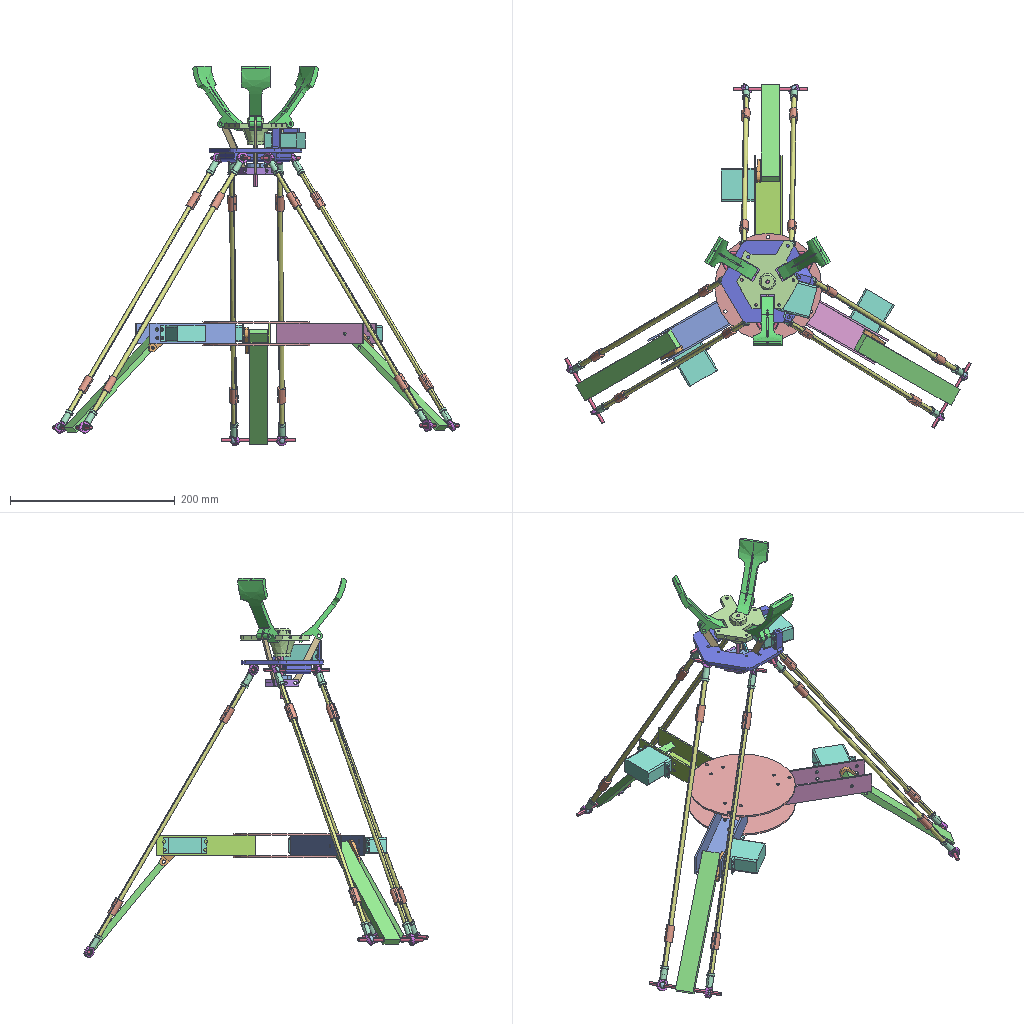Assembly | SolidWorks | 21 different items | 85 placed | box 494 x 418 x 460 mm
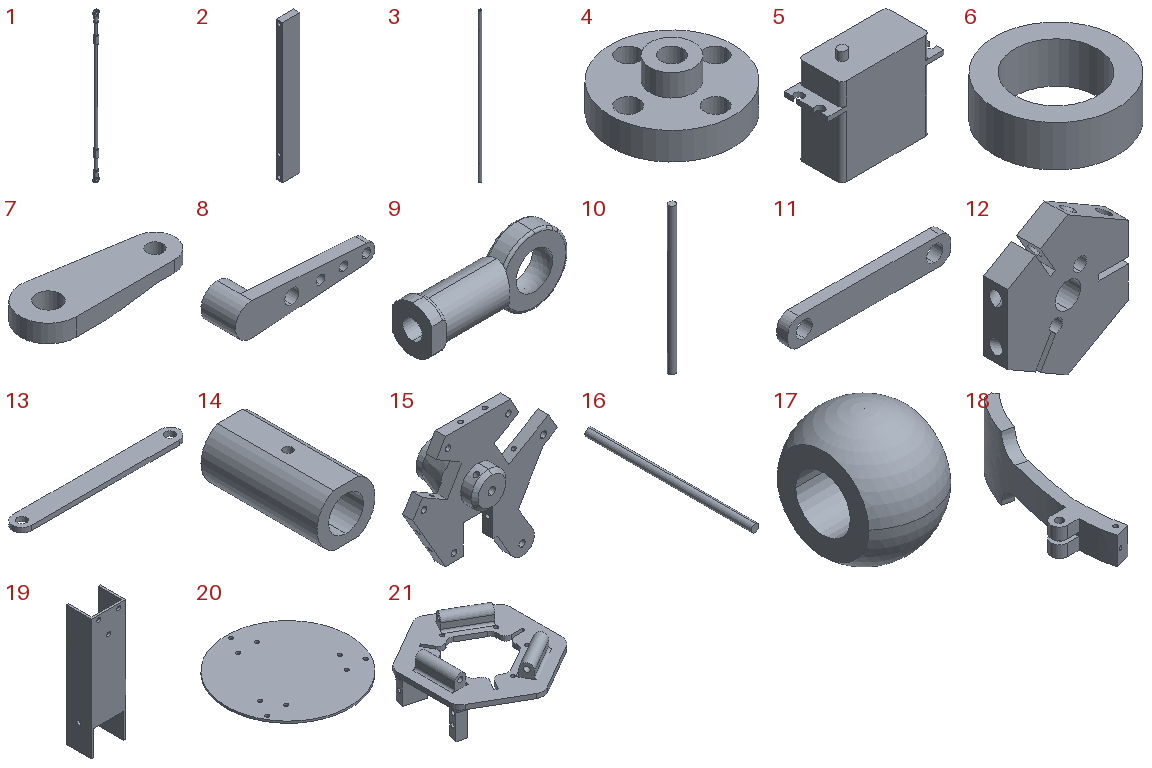Parts list (item | name | quantity | parent item | size | volume | features):
1 | (subassembly) | x6 | - | 14 x 10 x 410 mm | 9649 mm3 | -
2 | - | x3 | - | 22 x 8 x 175 mm | 29971 mm3 | features Extrusion 1, ICE 1
3 | - | x6 | in 1 | 6 x 6 x 350 mm | 5491 mm3 | features Extrusion 1, ICE 1
4 | - | x1 | - | 22.5 x 22.5 x 9 mm | 1758 mm3 | features ICE 2, Extrusion 1
5 | - | x4 | - | 53 x 20 x 44 mm | 32345 mm3 | features ICE 3, Extrusion 1, Fillet 1, MirrorPattern 1
6 | - | x3 | - | 6 x 6 x 2 mm | 31.416 mm3 | features Extrusion 1
7 | - | x3 | - | 36.997 x 14.091 x 4.508 mm | 1473 mm3 | features Extrusion 1, ICE 1
8 | - | x1 | - | 24.35 x 6 x 5.701 mm | 238.009 mm3 | features ICE 2, Extrusion 1
9 | - | x12 | in 1 | 30 x 8 x 14 mm | 1138 mm3 | features Fillet 3, ICE 3, Extrusion 1, RevCut 1
10 | - | x6 | - | 4 x 4 x 90 mm | 1131 mm3 | features Extrusion 1
11 | - | x1 | - | 30 x 2 x 5 mm | 264.858 mm3 | features Extrusion 1
12 | - | x1 | - | 40 x 8 x 46.188 mm | 8880 mm3 | features ICE 3, CirPattern 2, Cut 1, Extrusion 1
13 | - | x3 | - | 72 x 8 x 2 mm | 1074 mm3 | features Extrusion 1
14 | - | x12 | in 1 | 10 x 20 x 9 mm | 941.197 mm3 | features Extrusion 1, ICE 1
15 | - | x1 | - | 83.855 x 34 x 82.22 mm | 30431 mm3 | features ICE 8, CirPattern 3, Chamfer 2, Cut 2, Extrusion 1
16 | - | x1 | - | 4 x 85 x 4 mm | 1068 mm3 | features Extrusion 1
17 | - | x12 | - | 6 x 9 x 9 mm | 249.757 mm3 | features ICE 2, Revolution 1
18 | - | x3 | - | 38.444 x 92.062 x 35 mm | 13126 mm3 | features ICE 6, Fillet 2, Chamfer 1, Extrusion 1, SweepCut 1
19 | - | x3 | - | 34 x 25 x 120 mm | 17574 mm3 | features ICE 3, Extrusion 1
20 | - | x2 | - | 130 x 130 x 2 mm | 26320 mm3 | features Extrusion 1, ICE 1
21 | - | x1 | - | 100 x 112.376 x 41 mm | 40931 mm3 | features ICE 8, Fillet 7, Cut 3, CirPattern 2, Extrusion 1, RefAxis 1
Mates (type | each side: item.copy, entity, surface, feature):
In the top assembly
Coincident | 20.1 face plane Boss-Extrude1 | 19.1 face plane
Concentric | 20.1 face cylinder Cut-Extrude1 | 19.1 face cylinder | 2 times
Coincident | 20.1 face plane Boss-Extrude1 | 19.2 face plane
Concentric | 20.1 face cylinder Cut-Extrude1 | 19.2 face cylinder | 2 times
Coincident | 20.1 face plane Boss-Extrude1 | 19.3 face plane
Concentric | 20.1 face cylinder Cut-Extrude1 | 19.3 face cylinder | 2 times
Concentric | 20.1 face cylinder Boss-Extrude1 | 20.2 face cylinder Boss-Extrude1
Coincident | 19.2 face plane | 20.2 face plane Boss-Extrude1
Concentric | 20.1 face cylinder Cut-Extrude1 | 20.2 face cylinder Cut-Extrude1
Coincident | 19.3 face plane | 5.1 face plane Boss-Extrude1
Concentric | 19.3 face cylinder | 5.1 face cylinder Boss-Extrude3
Parallel | 19.3 face plane | 5.1 face plane Boss-Extrude1
Concentric | 19.2 face cylinder | 5.2 face cylinder Boss-Extrude3
Coincident | 19.2 face plane | 5.2 face plane Boss-Extrude1
Parallel | 19.2 face plane | 5.2 face plane Boss-Extrude1
Concentric | 19.1 face cylinder | 5.3 face cylinder Boss-Extrude3
Coincident | 19.1 face plane | 5.3 face plane Boss-Extrude1
Parallel | 19.1 face plane | 5.3 face plane Boss-Extrude1
Concentric | 5.2 face cylinder Boss-Extrude3 | 6.1 face cylinder Boss-Extrude1
Coincident | 19.2 face plane | 6.1 face plane Boss-Extrude1
Concentric | 5.3 face cylinder Boss-Extrude3 | 6.2 face cylinder Boss-Extrude1
Coincident | 19.1 face plane | 6.2 face plane Boss-Extrude1
Concentric | 5.1 face cylinder Boss-Extrude3 | 6.3 face cylinder Boss-Extrude1
Coincident | 19.3 face plane | 6.3 face plane Boss-Extrude1
Concentric | 7.1 face cylinder Boss-Extrude1 | 6.1 face cylinder Boss-Extrude1
DistanceDim | 19.2 face plane | 7.1 face plane Cut-Extrude1
Concentric | 7.1 face cylinder Boss-Extrude1 | 2.1 face cylinder Cut-Extrude1 | 2 times
DistanceDim | 7.1 face plane Boss-Extrude1 | 2.1 face plane Boss-Extrude1
Concentric | 6.3 face cylinder Boss-Extrude1 | 7.2 face cylinder Boss-Extrude1
DistanceDim | 19.3 face plane | 7.2 face plane Cut-Extrude1
Concentric | 2.2 face cylinder Cut-Extrude1 | 7.2 face cylinder Boss-Extrude1 | 2 times
DistanceDim | 2.2 face plane Boss-Extrude1 | 7.2 face plane Boss-Extrude1
Concentric | 6.2 face cylinder Boss-Extrude1 | 7.3 face cylinder Boss-Extrude1
DistanceDim | 7.3 face plane Cut-Extrude1 | 19.1 face plane
Concentric | 2.3 face cylinder Cut-Extrude1 | 7.3 face cylinder Boss-Extrude1 | 2 times
DistanceDim | 2.3 face plane Boss-Extrude1 | 7.3 face plane Boss-Extrude1
Concentric | 2.1 face cylinder Cut-Extrude1 | 10.1 face cylinder Boss-Extrude1
Width | 2.1 face plane Boss-Extrude1 | 2.1 face plane Boss-Extrude1 | 10.1 face plane Boss-Extrude1 | 10.1 face plane Boss-Extrude1
Concentric | 2.3 face cylinder Cut-Extrude1 | 10.2 face cylinder Boss-Extrude1
DistanceDim | 2.3 face plane Boss-Extrude1 | 10.2 face plane Boss-Extrude1
Concentric | 2.2 face cylinder Cut-Extrude1 | 10.3 face cylinder Boss-Extrude1
DistanceDim | 2.2 face plane Boss-Extrude1 | 10.3 face plane Boss-Extrude1
Concentric | 10.2 face cylinder Boss-Extrude1 | 17.1 face cylinder Cut-Extrude3
DistanceDim | 17.1 face plane Cut-Extrude2 | 2.3 face plane Boss-Extrude1
Concentric | 10.2 face cylinder Boss-Extrude1 | 17.2 face cylinder Cut-Extrude3
DistanceDim | 2.3 face plane Boss-Extrude1 | 17.2 face plane Cut-Extrude2
Concentric | 10.1 face cylinder Boss-Extrude1 | 17.3 face cylinder Cut-Extrude3
DistanceDim | 17.3 face plane Cut-Extrude2 | 2.1 face plane Boss-Extrude1
Concentric | 10.1 face cylinder Boss-Extrude1 | 17.4 face cylinder Cut-Extrude3
DistanceDim | 17.4 face plane Cut-Extrude2 | 2.1 face plane Boss-Extrude1
Concentric | 10.3 face cylinder Boss-Extrude1 | 17.5 face cylinder Cut-Extrude3
DistanceDim | 2.2 face plane Boss-Extrude1 | 17.5 face plane Cut-Extrude2
Concentric | 10.3 face cylinder Boss-Extrude1 | 17.6 face cylinder Cut-Extrude3
DistanceDim | 2.2 face plane Boss-Extrude1 | 17.6 face plane Cut-Extrude2
Concentric | 17.2 face sphere Revolve4 | 9.1 face sphere Cut-Revolve3
Concentric | 17.1 face sphere Revolve4 | 9.2 face sphere Cut-Revolve3
Concentric | 17.3 face sphere Revolve4 | 9.3 face sphere Cut-Revolve3
Concentric | 17.4 face sphere Revolve4 | 9.4 face sphere Cut-Revolve3
Concentric | 17.6 face sphere Revolve4 | 9.5 face sphere Cut-Revolve3
Concentric | 17.5 face sphere Revolve4 | 9.6 face sphere Cut-Revolve3
Parallel | 20.1 face plane Boss-Extrude1 | 21.1 face plane Boss-Extrude1
Concentric | 21.1 face cylinder CirPattern1 | 10.4 face cylinder Boss-Extrude1
Width | 21.1 face plane CirPattern1 | 21.1 face plane CirPattern1 | 10.4 face plane Boss-Extrude1 | 10.4 face plane Boss-Extrude1
Concentric | 10.5 face cylinder Boss-Extrude1 | 21.1 face cylinder Boss-Extrude2
DistanceDim | 21.1 face plane Boss-Extrude2 | 10.5 face plane Boss-Extrude1
Concentric | 21.1 face cylinder CirPattern1 | 10.6 face cylinder Boss-Extrude1
DistanceDim | 10.6 face plane Boss-Extrude1 | 21.1 face plane CirPattern1
Concentric | 10.6 face cylinder Boss-Extrude1 | 17.7 face cylinder Cut-Extrude3
DistanceDim | 17.7 face plane Cut-Extrude2 | 10.6 face plane Boss-Extrude1
Concentric | 10.6 face cylinder Boss-Extrude1 | 17.8 face cylinder Cut-Extrude3
DistanceDim | 17.8 face plane Cut-Extrude2 | 10.6 face plane Boss-Extrude1
Concentric | 10.4 face cylinder Boss-Extrude1 | 17.9 face cylinder Cut-Extrude3
DistanceDim | 17.9 face plane Cut-Extrude2 | 10.4 face plane Boss-Extrude1
Concentric | 10.4 face cylinder Boss-Extrude1 | 17.10 face cylinder Cut-Extrude3
DistanceDim | 17.10 face plane Cut-Extrude2 | 10.4 face plane Boss-Extrude1
Concentric | 10.5 face cylinder Boss-Extrude1 | 17.11 face cylinder Cut-Extrude3
Concentric | 10.5 face cylinder Boss-Extrude1 | 17.12 face cylinder Cut-Extrude3
DistanceDim | 17.11 face plane Cut-Extrude2 | 10.5 face plane Boss-Extrude1
DistanceDim | 17.12 face plane Cut-Extrude2 | 10.5 face plane Boss-Extrude1
Concentric | 9.7 face sphere Cut-Revolve3 | 17.8 face sphere Revolve4
Concentric | 9.8 face sphere Cut-Revolve3 | 17.7 face sphere Revolve4
Concentric | 9.9 face sphere Cut-Revolve3 | 17.9 face sphere Revolve4
Concentric | 9.10 face sphere Cut-Revolve3 | 17.10 face sphere Revolve4
Concentric | 9.11 face sphere Cut-Revolve3 | 17.11 face sphere Revolve4
Concentric | 9.12 face sphere Cut-Revolve3 | 17.12 face sphere Revolve4
Coincident | 21.1 face plane Boss-Extrude1 | 5.4 face plane Boss-Extrude1
Concentric | 21.1 face cylinder Cut-Extrude7 | 5.4 face cylinder Cut-Extrude1
Concentric | 21.1 face cylinder Cut-Extrude7 | 5.4 face cylinder Mirror2
Coincident | 21.1 face plane Boss-Extrude4 | 5.4 face plane Boss-Extrude2
Concentric | 15.1 face cylinder Cut-Extrude1 | 16.1 face cylinder Boss-Extrude1
Coincident | 15.1 face plane Boss-Extrude3 | 16.1 face plane Boss-Extrude1
Concentric | 15.1 face cylinder CirPattern1 | 18.1 face cylinder Cut-Extrude1
DistanceDim | 18.1 face plane Boss-Extrude1 | 15.1 face plane Boss-Extrude1
Concentric | 15.1 face cylinder CirPattern1 | 18.2 face cylinder Cut-Extrude1
DistanceDim | 18.2 face plane Boss-Extrude1 | 15.1 face plane Boss-Extrude1
Concentric | 15.1 face cylinder Cut-Extrude2 | 18.3 face cylinder Cut-Extrude1
DistanceDim | 18.3 face plane Boss-Extrude1 | 15.1 face plane Boss-Extrude1
Concentric | 13.1 face cylinder Boss-Extrude1 | 18.2 face cylinder Boss-Extrude2
Coincident | 13.1 face plane Boss-Extrude1 | 18.2 face plane Cut-Extrude2
Concentric | 18.1 face cylinder Boss-Extrude2 | 13.2 face cylinder Boss-Extrude1
Coincident | 18.1 face plane Cut-Extrude2 | 13.2 face plane Boss-Extrude1
Concentric | 18.3 face cylinder Boss-Extrude2 | 13.3 face cylinder Boss-Extrude1
Coincident | 18.3 face plane Cut-Extrude2 | 13.3 face plane Boss-Extrude1
Concentric | 16.1 face cylinder Boss-Extrude1 | 12.1 face cylinder Cut-Extrude1
Concentric | 12.1 face cylinder Cut-Extrude4 | 13.3 face cylinder Boss-Extrude1
Concentric | 12.1 face cylinder CirPattern2 | 13.2 face cylinder Boss-Extrude1
Concentric | 13.1 face cylinder Boss-Extrude1 | 12.1 face cylinder CirPattern2
Concentric | 5.4 face cylinder Boss-Extrude3 | 8.1 face cylinder Boss-Extrude2
Coincident | 5.4 face plane Boss-Extrude1 | 8.1 face plane Boss-Extrude2
Concentric | 11.1 face cylinder Boss-Extrude1 | 8.1 face cylinder Cut-Extrude1
Coincident | 11.1 face plane Boss-Extrude1 | 8.1 face plane Boss-Extrude1
Concentric | 16.1 face cylinder Boss-Extrude1 | 4.1 face cylinder Boss-Extrude1
Coincident | 12.1 face plane Boss-Extrude1 | 4.1 face plane Boss-Extrude1
Parallel | 21.1 face plane Boss-Extrude1 | 12.1 face plane Boss-Extrude1
Concentric | 21.1 select_type:24 | 16.1 face cylinder Boss-Extrude1
Concentric | 11.1 face cylinder Boss-Extrude1 | 4.1 face cylinder Cut-Extrude1
Parallel | 21.1 face plane CirPattern2 | 13.1 face plane Boss-Extrude1
DistanceDim | 15.1 face plane Boss-Extrude1 | 21.1 face plane Boss-Extrude1
In subassembly 1
Concentric | 3.1 face cylinder Boss-Extrude1 | 9.13 face cylinder Cut-Extrude1
Coincident | 3.1 face plane Boss-Extrude1 | 9.13 face plane Boss-Extrude2
Concentric | 3.1 face cylinder Boss-Extrude1 | 9.14 face cylinder Cut-Extrude1
Coincident | 3.1 face plane Boss-Extrude1 | 9.14 face plane Boss-Extrude2
Concentric | 3.1 face cylinder Boss-Extrude1 | 14.1 face cylinder Boss-Extrude1
Concentric | 3.1 face cylinder Cut-Extrude1 | 14.1 face cylinder Cut-Extrude1
Concentric | 3.1 face cylinder Boss-Extrude1 | 14.2 face cylinder Boss-Extrude1
Concentric | 3.1 face cylinder Cut-Extrude1 | 14.2 face cylinder Cut-Extrude1
Perpendicular | 9.14 face plane Boss-Extrude1 | 14.1 face plane Boss-Extrude1
Perpendicular | 9.13 face plane Boss-Extrude1 | 14.2 face plane Boss-Extrude1